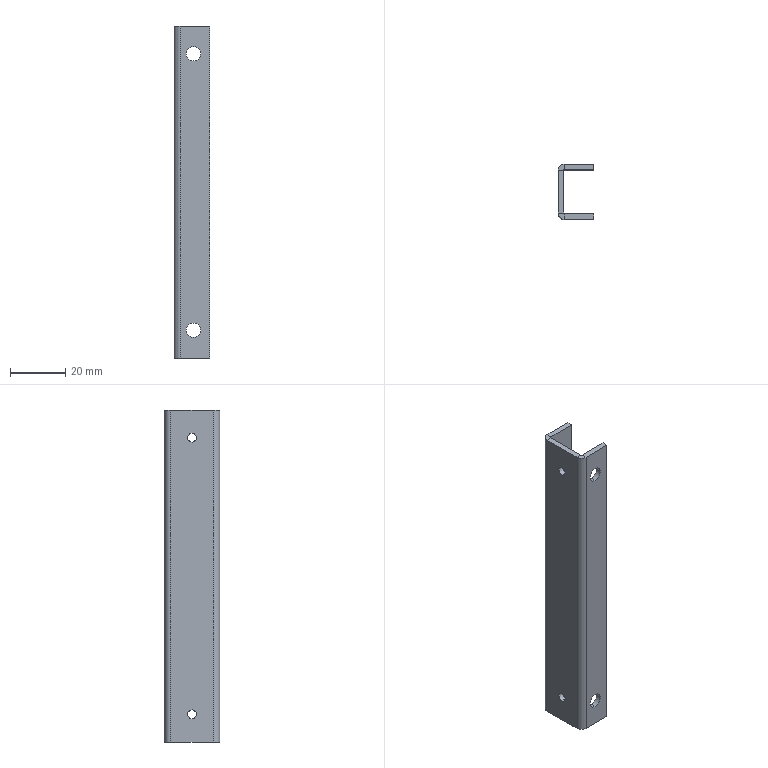Part | SolidWorks | features Cut 2, FlatPattern 1, SMBaseFlange 1, SheetMetal 1 | 1 solid | 34 faces | box 13 x 20 x 120 mm | volume 9610 mm3 | plane 18 | cylinder 16 | commonest cylinder face diameters 5.2 x8 3.2 x4 0.6 x2 4.6 x2
STEP:
#1=CARTESIAN_POINT('',(7.,18.,7.4));
#2=VERTEX_POINT('',#1);
#3=CARTESIAN_POINT('',(7.,18.,12.6));
#4=VERTEX_POINT('',#3);
#5=CARTESIAN_POINT('',(7.,18.,10.));
#6=DIRECTION('',(0.,1.,0.));
#7=DIRECTION('',(0.,0.,1.));
#8=AXIS2_PLACEMENT_3D('',#5,#6,#7);
#9=CIRCLE('',#8,2.6);
#10=EDGE_CURVE('',#2,#4,#9,.T.);
#11=ORIENTED_EDGE('',*,*,#10,.F.);
#12=CARTESIAN_POINT('',(7.,20.,7.4));
#13=VERTEX_POINT('',#12);
#14=CARTESIAN_POINT('',(7.,0.,7.4));
#15=DIRECTION('',(0.,1.,0.));
#16=VECTOR('',#15,1000.);
#17=LINE('',#14,#16);
#18=EDGE_CURVE('',#2,#13,#17,.T.);
#19=ORIENTED_EDGE('',*,*,#18,.T.);
#20=CARTESIAN_POINT('',(7.,20.,12.6));
#21=VERTEX_POINT('',#20);
#22=CARTESIAN_POINT('',(7.,20.,10.));
#23=DIRECTION('',(0.,1.,0.));
#24=DIRECTION('',(0.,0.,1.));
#25=AXIS2_PLACEMENT_3D('',#22,#23,#24);
#26=CIRCLE('',#25,2.6);
#27=EDGE_CURVE('',#13,#21,#26,.T.);
#28=ORIENTED_EDGE('',*,*,#27,.T.);
#29=CARTESIAN_POINT('',(7.,0.,12.6));
#30=DIRECTION('',(0.,1.,0.));
#31=VECTOR('',#30,1000.);
#32=LINE('',#29,#31);
#33=EDGE_CURVE('',#4,#21,#32,.T.);
#34=ORIENTED_EDGE('',*,*,#33,.F.);
#35=EDGE_LOOP('',(#11,#19,#28,#34));
#36=FACE_OUTER_BOUND('',#35,.T.);
#37=CARTESIAN_POINT('',(7.,0.,10.));
#38=DIRECTION('',(0.,1.,0.));
#39=DIRECTION('',(0.,0.,1.));
#40=AXIS2_PLACEMENT_3D('',#37,#38,#39);
#41=CYLINDRICAL_SURFACE('',#40,2.6);
#42=ADVANCED_FACE('',(#36),#41,.F.);
#43=CARTESIAN_POINT('',(7.,0.,7.4));
#44=VERTEX_POINT('',#43);
#45=CARTESIAN_POINT('',(7.,0.,12.6));
#46=VERTEX_POINT('',#45);
#47=CARTESIAN_POINT('',(7.,0.,10.));
#48=DIRECTION('',(0.,1.,0.));
#49=DIRECTION('',(0.,0.,1.));
#50=AXIS2_PLACEMENT_3D('',#47,#48,#49);
#51=CIRCLE('',#50,2.6);
#52=EDGE_CURVE('',#44,#46,#51,.T.);
#53=ORIENTED_EDGE('',*,*,#52,.F.);
#54=CARTESIAN_POINT('',(7.,2.,7.4));
#55=VERTEX_POINT('',#54);
#56=CARTESIAN_POINT('',(7.,0.,7.4));
#57=DIRECTION('',(0.,1.,0.));
#58=VECTOR('',#57,1000.);
#59=LINE('',#56,#58);
#60=EDGE_CURVE('',#44,#55,#59,.T.);
#61=ORIENTED_EDGE('',*,*,#60,.T.);
#62=CARTESIAN_POINT('',(7.,2.,12.6));
#63=VERTEX_POINT('',#62);
#64=CARTESIAN_POINT('',(7.,2.,10.));
#65=DIRECTION('',(0.,-1.,0.));
#66=DIRECTION('',(1.,0.,0.));
#67=AXIS2_PLACEMENT_3D('',#64,#65,#66);
#68=CIRCLE('',#67,2.6);
#69=EDGE_CURVE('',#63,#55,#68,.T.);
#70=ORIENTED_EDGE('',*,*,#69,.F.);
#71=CARTESIAN_POINT('',(7.,0.,12.6));
#72=DIRECTION('',(0.,1.,0.));
#73=VECTOR('',#72,1000.);
#74=LINE('',#71,#73);
#75=EDGE_CURVE('',#46,#63,#74,.T.);
#76=ORIENTED_EDGE('',*,*,#75,.F.);
#77=EDGE_LOOP('',(#53,#61,#70,#76));
#78=FACE_OUTER_BOUND('',#77,.T.);
#79=CARTESIAN_POINT('',(7.,0.,10.));
#80=DIRECTION('',(0.,1.,0.));
#81=DIRECTION('',(0.,0.,1.));
#82=AXIS2_PLACEMENT_3D('',#79,#80,#81);
#83=CYLINDRICAL_SURFACE('',#82,2.6);
#84=ADVANCED_FACE('',(#78),#83,.F.);
#85=CARTESIAN_POINT('',(7.,18.,107.4));
#86=VERTEX_POINT('',#85);
#87=CARTESIAN_POINT('',(7.,18.,112.6));
#88=VERTEX_POINT('',#87);
#89=CARTESIAN_POINT('',(7.,18.,110.));
#90=DIRECTION('',(0.,1.,0.));
#91=DIRECTION('',(0.,0.,1.));
#92=AXIS2_PLACEMENT_3D('',#89,#90,#91);
#93=CIRCLE('',#92,2.6);
#94=EDGE_CURVE('',#86,#88,#93,.T.);
#95=ORIENTED_EDGE('',*,*,#94,.F.);
#96=CARTESIAN_POINT('',(7.,20.,107.4));
#97=VERTEX_POINT('',#96);
#98=CARTESIAN_POINT('',(7.,0.,107.4));
#99=DIRECTION('',(0.,1.,0.));
#100=VECTOR('',#99,1000.);
#101=LINE('',#98,#100);
#102=EDGE_CURVE('',#86,#97,#101,.T.);
#103=ORIENTED_EDGE('',*,*,#102,.T.);
#104=CARTESIAN_POINT('',(7.,20.,112.6));
#105=VERTEX_POINT('',#104);
#106=CARTESIAN_POINT('',(7.,20.,110.));
#107=DIRECTION('',(0.,1.,0.));
#108=DIRECTION('',(0.,0.,1.));
#109=AXIS2_PLACEMENT_3D('',#106,#107,#108);
#110=CIRCLE('',#109,2.6);
#111=EDGE_CURVE('',#97,#105,#110,.T.);
#112=ORIENTED_EDGE('',*,*,#111,.T.);
#113=CARTESIAN_POINT('',(7.,0.,112.6));
#114=DIRECTION('',(0.,1.,0.));
#115=VECTOR('',#114,1000.);
#116=LINE('',#113,#115);
#117=EDGE_CURVE('',#88,#105,#116,.T.);
#118=ORIENTED_EDGE('',*,*,#117,.F.);
#119=EDGE_LOOP('',(#95,#103,#112,#118));
#120=FACE_OUTER_BOUND('',#119,.T.);
#121=CARTESIAN_POINT('',(7.,0.,110.));
#122=DIRECTION('',(0.,1.,0.));
#123=DIRECTION('',(0.,0.,1.));
#124=AXIS2_PLACEMENT_3D('',#121,#122,#123);
#125=CYLINDRICAL_SURFACE('',#124,2.6);
#126=ADVANCED_FACE('',(#120),#125,.F.);
#127=CARTESIAN_POINT('',(7.,0.,107.4));
#128=VERTEX_POINT('',#127);
#129=CARTESIAN_POINT('',(7.,0.,112.6));
#130=VERTEX_POINT('',#129);
#131=CARTESIAN_POINT('',(7.,0.,110.));
#132=DIRECTION('',(0.,1.,0.));
#133=DIRECTION('',(0.,0.,1.));
#134=AXIS2_PLACEMENT_3D('',#131,#132,#133);
#135=CIRCLE('',#134,2.6);
#136=EDGE_CURVE('',#128,#130,#135,.T.);
#137=ORIENTED_EDGE('',*,*,#136,.F.);
#138=CARTESIAN_POINT('',(7.,2.,107.4));
#139=VERTEX_POINT('',#138);
#140=CARTESIAN_POINT('',(7.,0.,107.4));
#141=DIRECTION('',(0.,1.,0.));
#142=VECTOR('',#141,1000.);
#143=LINE('',#140,#142);
#144=EDGE_CURVE('',#128,#139,#143,.T.);
#145=ORIENTED_EDGE('',*,*,#144,.T.);
#146=CARTESIAN_POINT('',(7.,2.,112.6));
#147=VERTEX_POINT('',#146);
#148=CARTESIAN_POINT('',(7.,2.,110.));
#149=DIRECTION('',(0.,-1.,0.));
#150=DIRECTION('',(1.,0.,0.));
#151=AXIS2_PLACEMENT_3D('',#148,#149,#150);
#152=CIRCLE('',#151,2.6);
#153=EDGE_CURVE('',#147,#139,#152,.T.);
#154=ORIENTED_EDGE('',*,*,#153,.F.);
#155=CARTESIAN_POINT('',(7.,0.,112.6));
#156=DIRECTION('',(0.,1.,0.));
#157=VECTOR('',#156,1000.);
#158=LINE('',#155,#157);
#159=EDGE_CURVE('',#130,#147,#158,.T.);
#160=ORIENTED_EDGE('',*,*,#159,.F.);
#161=EDGE_LOOP('',(#137,#145,#154,#160));
#162=FACE_OUTER_BOUND('',#161,.T.);
#163=CARTESIAN_POINT('',(7.,0.,110.));
#164=DIRECTION('',(0.,1.,0.));
#165=DIRECTION('',(0.,0.,1.));
#166=AXIS2_PLACEMENT_3D('',#163,#164,#165);
#167=CYLINDRICAL_SURFACE('',#166,2.6);
#168=ADVANCED_FACE('',(#162),#167,.F.);
#169=CARTESIAN_POINT('',(2.,10.,108.4));
#170=VERTEX_POINT('',#169);
#171=CARTESIAN_POINT('',(2.,10.,111.6));
#172=VERTEX_POINT('',#171);
#173=CARTESIAN_POINT('',(2.,10.,110.));
#174=DIRECTION('',(-1.,0.,0.));
#175=DIRECTION('',(0.,0.,1.));
#176=AXIS2_PLACEMENT_3D('',#173,#174,#175);
#177=CIRCLE('',#176,1.6);
#178=EDGE_CURVE('',#170,#172,#177,.T.);
#179=ORIENTED_EDGE('',*,*,#178,.F.);
#180=CARTESIAN_POINT('',(0.,10.,108.4));
#181=VERTEX_POINT('',#180);
#182=CARTESIAN_POINT('',(2.,10.,108.4));
#183=DIRECTION('',(-1.,0.,0.));
#184=VECTOR('',#183,1000.);
#185=LINE('',#182,#184);
#186=EDGE_CURVE('',#170,#181,#185,.T.);
#187=ORIENTED_EDGE('',*,*,#186,.T.);
#188=CARTESIAN_POINT('',(0.,10.,111.6));
#189=VERTEX_POINT('',#188);
#190=CARTESIAN_POINT('',(0.,10.,110.));
#191=DIRECTION('',(-1.,0.,0.));
#192=DIRECTION('',(0.,0.,1.));
#193=AXIS2_PLACEMENT_3D('',#190,#191,#192);
#194=CIRCLE('',#193,1.6);
#195=EDGE_CURVE('',#181,#189,#194,.T.);
#196=ORIENTED_EDGE('',*,*,#195,.T.);
#197=CARTESIAN_POINT('',(2.,10.,111.6));
#198=DIRECTION('',(-1.,0.,0.));
#199=VECTOR('',#198,1000.);
#200=LINE('',#197,#199);
#201=EDGE_CURVE('',#172,#189,#200,.T.);
#202=ORIENTED_EDGE('',*,*,#201,.F.);
#203=EDGE_LOOP('',(#179,#187,#196,#202));
#204=FACE_OUTER_BOUND('',#203,.T.);
#205=CARTESIAN_POINT('',(2.,10.,110.));
#206=DIRECTION('',(-1.,0.,0.));
#207=DIRECTION('',(0.,0.,1.));
#208=AXIS2_PLACEMENT_3D('',#205,#206,#207);
#209=CYLINDRICAL_SURFACE('',#208,1.6);
#210=ADVANCED_FACE('',(#204),#209,.F.);
#211=CARTESIAN_POINT('',(2.,10.,8.4));
#212=VERTEX_POINT('',#211);
#213=CARTESIAN_POINT('',(2.,10.,11.6));
#214=VERTEX_POINT('',#213);
#215=CARTESIAN_POINT('',(2.,10.,10.));
#216=DIRECTION('',(-1.,0.,0.));
#217=DIRECTION('',(0.,0.,1.));
#218=AXIS2_PLACEMENT_3D('',#215,#216,#217);
#219=CIRCLE('',#218,1.6);
#220=EDGE_CURVE('',#212,#214,#219,.T.);
#221=ORIENTED_EDGE('',*,*,#220,.F.);
#222=CARTESIAN_POINT('',(0.,10.,8.4));
#223=VERTEX_POINT('',#222);
#224=CARTESIAN_POINT('',(2.,10.,8.4));
#225=DIRECTION('',(-1.,0.,0.));
#226=VECTOR('',#225,1000.);
#227=LINE('',#224,#226);
#228=EDGE_CURVE('',#212,#223,#227,.T.);
#229=ORIENTED_EDGE('',*,*,#228,.T.);
#230=CARTESIAN_POINT('',(0.,10.,11.6));
#231=VERTEX_POINT('',#230);
#232=CARTESIAN_POINT('',(0.,10.,10.));
#233=DIRECTION('',(-1.,0.,0.));
#234=DIRECTION('',(0.,0.,1.));
#235=AXIS2_PLACEMENT_3D('',#232,#233,#234);
#236=CIRCLE('',#235,1.6);
#237=EDGE_CURVE('',#223,#231,#236,.T.);
#238=ORIENTED_EDGE('',*,*,#237,.T.);
#239=CARTESIAN_POINT('',(2.,10.,11.6));
#240=DIRECTION('',(-1.,0.,0.));
#241=VECTOR('',#240,1000.);
#242=LINE('',#239,#241);
#243=EDGE_CURVE('',#214,#231,#242,.T.);
#244=ORIENTED_EDGE('',*,*,#243,.F.);
#245=EDGE_LOOP('',(#221,#229,#238,#244));
#246=FACE_OUTER_BOUND('',#245,.T.);
#247=CARTESIAN_POINT('',(2.,10.,10.));
#248=DIRECTION('',(-1.,0.,0.));
#249=DIRECTION('',(0.,0.,1.));
#250=AXIS2_PLACEMENT_3D('',#247,#248,#249);
#251=CYLINDRICAL_SURFACE('',#250,1.6);
#252=ADVANCED_FACE('',(#246),#251,.F.);
#253=CARTESIAN_POINT('',(0.,2.3,120.));
#254=VERTEX_POINT('',#253);
#255=CARTESIAN_POINT('',(2.,2.3,120.));
#256=VERTEX_POINT('',#255);
#257=CARTESIAN_POINT('',(0.,2.3,120.));
#258=DIRECTION('',(1.,0.,0.));
#259=VECTOR('',#258,1000.);
#260=LINE('',#257,#259);
#261=EDGE_CURVE('',#254,#256,#260,.T.);
#262=ORIENTED_EDGE('',*,*,#261,.F.);
#263=CARTESIAN_POINT('',(2.3,0.,120.));
#264=VERTEX_POINT('',#263);
#265=CARTESIAN_POINT('',(2.3,2.3,120.));
#266=DIRECTION('',(0.,0.,-1.));
#267=DIRECTION('',(1.,0.,0.));
#268=AXIS2_PLACEMENT_3D('',#265,#266,#267);
#269=CIRCLE('',#268,2.3);
#270=EDGE_CURVE('',#264,#254,#269,.T.);
#271=ORIENTED_EDGE('',*,*,#270,.F.);
#272=CARTESIAN_POINT('',(2.3,2.,120.));
#273=VERTEX_POINT('',#272);
#274=CARTESIAN_POINT('',(2.3,2.,120.));
#275=DIRECTION('',(0.,-1.,0.));
#276=VECTOR('',#275,1000.);
#277=LINE('',#274,#276);
#278=EDGE_CURVE('',#273,#264,#277,.T.);
#279=ORIENTED_EDGE('',*,*,#278,.F.);
#280=CARTESIAN_POINT('',(2.3,2.3,120.));
#281=DIRECTION('',(0.,0.,-1.));
#282=DIRECTION('',(1.,0.,0.));
#283=AXIS2_PLACEMENT_3D('',#280,#281,#282);
#284=CIRCLE('',#283,0.3);
#285=EDGE_CURVE('',#273,#256,#284,.T.);
#286=ORIENTED_EDGE('',*,*,#285,.T.);
#287=EDGE_LOOP('',(#262,#271,#279,#286));
#288=FACE_OUTER_BOUND('',#287,.T.);
#289=CARTESIAN_POINT('',(0.,2.3,120.));
#290=DIRECTION('',(0.,0.,1.));
#291=DIRECTION('',(1.,0.,0.));
#292=AXIS2_PLACEMENT_3D('',#289,#290,#291);
#293=PLANE('',#292);
#294=ADVANCED_FACE('',(#288),#293,.T.);
#295=CARTESIAN_POINT('',(0.,17.7,120.));
#296=VERTEX_POINT('',#295);
#297=CARTESIAN_POINT('',(0.,0.,120.));
#298=DIRECTION('',(0.,1.,0.));
#299=VECTOR('',#298,1000.);
#300=LINE('',#297,#299);
#301=EDGE_CURVE('',#254,#296,#300,.T.);
#302=ORIENTED_EDGE('',*,*,#301,.F.);
#303=ORIENTED_EDGE('',*,*,#261,.T.);
#304=CARTESIAN_POINT('',(2.,17.7,120.));
#305=VERTEX_POINT('',#304);
#306=CARTESIAN_POINT('',(2.,0.,120.));
#307=DIRECTION('',(0.,1.,0.));
#308=VECTOR('',#307,1000.);
#309=LINE('',#306,#308);
#310=EDGE_CURVE('',#256,#305,#309,.T.);
#311=ORIENTED_EDGE('',*,*,#310,.T.);
#312=CARTESIAN_POINT('',(2.,17.7,120.));
#313=DIRECTION('',(-1.,0.,0.));
#314=VECTOR('',#313,1000.);
#315=LINE('',#312,#314);
#316=EDGE_CURVE('',#305,#296,#315,.T.);
#317=ORIENTED_EDGE('',*,*,#316,.T.);
#318=EDGE_LOOP('',(#302,#303,#311,#317));
#319=FACE_OUTER_BOUND('',#318,.T.);
#320=CARTESIAN_POINT('',(2.3,2.,120.));
#321=DIRECTION('',(0.,0.,1.));
#322=DIRECTION('',(1.,0.,0.));
#323=AXIS2_PLACEMENT_3D('',#320,#321,#322);
#324=PLANE('',#323);
#325=ADVANCED_FACE('',(#319),#324,.T.);
#326=CARTESIAN_POINT('',(2.3,0.,0.));
#327=VERTEX_POINT('',#326);
#328=CARTESIAN_POINT('',(2.3,2.,0.));
#329=VERTEX_POINT('',#328);
#330=CARTESIAN_POINT('',(2.3,0.,0.));
#331=DIRECTION('',(0.,1.,0.));
#332=VECTOR('',#331,1000.);
#333=LINE('',#330,#332);
#334=EDGE_CURVE('',#327,#329,#333,.T.);
#335=ORIENTED_EDGE('',*,*,#334,.F.);
#336=CARTESIAN_POINT('',(0.,2.3,0.));
#337=VERTEX_POINT('',#336);
#338=CARTESIAN_POINT('',(2.3,2.3,0.));
#339=DIRECTION('',(0.,0.,-1.));
#340=DIRECTION('',(1.,0.,0.));
#341=AXIS2_PLACEMENT_3D('',#338,#339,#340);
#342=CIRCLE('',#341,2.3);
#343=EDGE_CURVE('',#327,#337,#342,.T.);
#344=ORIENTED_EDGE('',*,*,#343,.T.);
#345=CARTESIAN_POINT('',(2.,2.3,0.));
#346=VERTEX_POINT('',#345);
#347=CARTESIAN_POINT('',(2.,2.3,0.));
#348=DIRECTION('',(-1.,0.,0.));
#349=VECTOR('',#348,1000.);
#350=LINE('',#347,#349);
#351=EDGE_CURVE('',#346,#337,#350,.T.);
#352=ORIENTED_EDGE('',*,*,#351,.F.);
#353=CARTESIAN_POINT('',(2.3,2.3,0.));
#354=DIRECTION('',(0.,0.,-1.));
#355=DIRECTION('',(1.,0.,0.));
#356=AXIS2_PLACEMENT_3D('',#353,#354,#355);
#357=CIRCLE('',#356,0.3);
#358=EDGE_CURVE('',#329,#346,#357,.T.);
#359=ORIENTED_EDGE('',*,*,#358,.F.);
#360=EDGE_LOOP('',(#335,#344,#352,#359));
#361=FACE_OUTER_BOUND('',#360,.T.);
#362=CARTESIAN_POINT('',(2.3,0.,0.));
#363=DIRECTION('',(0.,0.,-1.));
#364=DIRECTION('',(-1.,0.,0.));
#365=AXIS2_PLACEMENT_3D('',#362,#363,#364);
#366=PLANE('',#365);
#367=ADVANCED_FACE('',(#361),#366,.T.);
#368=CARTESIAN_POINT('',(13.,0.,0.));
#369=VERTEX_POINT('',#368);
#370=CARTESIAN_POINT('',(13.,0.,0.));
#371=DIRECTION('',(-1.,0.,0.));
#372=VECTOR('',#371,1000.);
#373=LINE('',#370,#372);
#374=EDGE_CURVE('',#369,#327,#373,.T.);
#375=ORIENTED_EDGE('',*,*,#374,.T.);
#376=ORIENTED_EDGE('',*,*,#334,.T.);
#377=CARTESIAN_POINT('',(13.,2.,0.));
#378=VERTEX_POINT('',#377);
#379=CARTESIAN_POINT('',(13.,2.,0.));
#380=DIRECTION('',(-1.,0.,0.));
#381=VECTOR('',#380,1000.);
#382=LINE('',#379,#381);
#383=EDGE_CURVE('',#378,#329,#382,.T.);
#384=ORIENTED_EDGE('',*,*,#383,.F.);
#385=CARTESIAN_POINT('',(13.,2.,0.));
#386=DIRECTION('',(0.,-1.,0.));
#387=VECTOR('',#386,1000.);
#388=LINE('',#385,#387);
#389=EDGE_CURVE('',#378,#369,#388,.T.);
#390=ORIENTED_EDGE('',*,*,#389,.T.);
#391=EDGE_LOOP('',(#375,#376,#384,#390));
#392=FACE_OUTER_BOUND('',#391,.T.);
#393=CARTESIAN_POINT('',(2.,2.3,0.));
#394=DIRECTION('',(0.,0.,-1.));
#395=DIRECTION('',(-1.,0.,0.));
#396=AXIS2_PLACEMENT_3D('',#393,#394,#395);
#397=PLANE('',#396);
#398=ADVANCED_FACE('',(#392),#397,.T.);
#399=CARTESIAN_POINT('',(2.3,20.,120.));
#400=VERTEX_POINT('',#399);
#401=CARTESIAN_POINT('',(2.3,18.,120.));
#402=VERTEX_POINT('',#401);
#403=CARTESIAN_POINT('',(2.3,20.,120.));
#404=DIRECTION('',(0.,-1.,0.));
#405=VECTOR('',#404,1000.);
#406=LINE('',#403,#405);
#407=EDGE_CURVE('',#400,#402,#406,.T.);
#408=ORIENTED_EDGE('',*,*,#407,.F.);
#409=CARTESIAN_POINT('',(2.3,17.7,120.));
#410=DIRECTION('',(0.,0.,-1.));
#411=DIRECTION('',(1.,0.,0.));
#412=AXIS2_PLACEMENT_3D('',#409,#410,#411);
#413=CIRCLE('',#412,2.3);
#414=EDGE_CURVE('',#296,#400,#413,.T.);
#415=ORIENTED_EDGE('',*,*,#414,.F.);
#416=ORIENTED_EDGE('',*,*,#316,.F.);
#417=CARTESIAN_POINT('',(2.3,17.7,120.));
#418=DIRECTION('',(0.,0.,-1.));
#419=DIRECTION('',(1.,0.,0.));
#420=AXIS2_PLACEMENT_3D('',#417,#418,#419);
#421=CIRCLE('',#420,0.3);
#422=EDGE_CURVE('',#305,#402,#421,.T.);
#423=ORIENTED_EDGE('',*,*,#422,.T.);
#424=EDGE_LOOP('',(#408,#415,#416,#423));
#425=FACE_OUTER_BOUND('',#424,.T.);
#426=CARTESIAN_POINT('',(2.3,20.,120.));
#427=DIRECTION('',(0.,0.,1.));
#428=DIRECTION('',(1.,0.,0.));
#429=AXIS2_PLACEMENT_3D('',#426,#427,#428);
#430=PLANE('',#429);
#431=ADVANCED_FACE('',(#425),#430,.T.);
#432=CARTESIAN_POINT('',(13.,20.,120.));
#433=VERTEX_POINT('',#432);
#434=CARTESIAN_POINT('',(0.,20.,120.));
#435=DIRECTION('',(1.,0.,0.));
#436=VECTOR('',#435,1000.);
#437=LINE('',#434,#436);
#438=EDGE_CURVE('',#400,#433,#437,.T.);
#439=ORIENTED_EDGE('',*,*,#438,.F.);
#440=ORIENTED_EDGE('',*,*,#407,.T.);
#441=CARTESIAN_POINT('',(13.,18.,120.));
#442=VERTEX_POINT('',#441);
#443=CARTESIAN_POINT('',(0.,18.,120.));
#444=DIRECTION('',(1.,0.,0.));
#445=VECTOR('',#444,1000.);
#446=LINE('',#443,#445);
#447=EDGE_CURVE('',#402,#442,#446,.T.);
#448=ORIENTED_EDGE('',*,*,#447,.T.);
#449=CARTESIAN_POINT('',(13.,20.,120.));
#450=DIRECTION('',(0.,-1.,0.));
#451=VECTOR('',#450,1000.);
#452=LINE('',#449,#451);
#453=EDGE_CURVE('',#433,#442,#452,.T.);
#454=ORIENTED_EDGE('',*,*,#453,.F.);
#455=EDGE_LOOP('',(#439,#440,#448,#454));
#456=FACE_OUTER_BOUND('',#455,.T.);
#457=CARTESIAN_POINT('',(2.,17.7,120.));
#458=DIRECTION('',(0.,0.,1.));
#459=DIRECTION('',(1.,0.,0.));
#460=AXIS2_PLACEMENT_3D('',#457,#458,#459);
#461=PLANE('',#460);
#462=ADVANCED_FACE('',(#456),#461,.T.);
#463=CARTESIAN_POINT('',(0.,17.7,0.));
#464=VERTEX_POINT('',#463);
#465=CARTESIAN_POINT('',(2.,17.7,0.));
#466=VERTEX_POINT('',#465);
#467=CARTESIAN_POINT('',(0.,17.7,0.));
#468=DIRECTION('',(1.,0.,0.));
#469=VECTOR('',#468,1000.);
#470=LINE('',#467,#469);
#471=EDGE_CURVE('',#464,#466,#470,.T.);
#472=ORIENTED_EDGE('',*,*,#471,.F.);
#473=CARTESIAN_POINT('',(2.3,20.,0.));
#474=VERTEX_POINT('',#473);
#475=CARTESIAN_POINT('',(2.3,17.7,0.));
#476=DIRECTION('',(0.,0.,-1.));
#477=DIRECTION('',(1.,0.,0.));
#478=AXIS2_PLACEMENT_3D('',#475,#476,#477);
#479=CIRCLE('',#478,2.3);
#480=EDGE_CURVE('',#464,#474,#479,.T.);
#481=ORIENTED_EDGE('',*,*,#480,.T.);
#482=CARTESIAN_POINT('',(2.3,18.,0.));
#483=VERTEX_POINT('',#482);
#484=CARTESIAN_POINT('',(2.3,18.,0.));
#485=DIRECTION('',(0.,1.,0.));
#486=VECTOR('',#485,1000.);
#487=LINE('',#484,#486);
#488=EDGE_CURVE('',#483,#474,#487,.T.);
#489=ORIENTED_EDGE('',*,*,#488,.F.);
#490=CARTESIAN_POINT('',(2.3,17.7,0.));
#491=DIRECTION('',(0.,0.,-1.));
#492=DIRECTION('',(1.,0.,0.));
#493=AXIS2_PLACEMENT_3D('',#490,#491,#492);
#494=CIRCLE('',#493,0.3);
#495=EDGE_CURVE('',#466,#483,#494,.T.);
#496=ORIENTED_EDGE('',*,*,#495,.F.);
#497=EDGE_LOOP('',(#472,#481,#489,#496));
#498=FACE_OUTER_BOUND('',#497,.T.);
#499=CARTESIAN_POINT('',(0.,17.7,0.));
#500=DIRECTION('',(0.,0.,-1.));
#501=DIRECTION('',(-1.,0.,0.));
#502=AXIS2_PLACEMENT_3D('',#499,#500,#501);
#503=PLANE('',#502);
#504=ADVANCED_FACE('',(#498),#503,.T.);
#505=CARTESIAN_POINT('',(0.,0.,0.));
#506=DIRECTION('',(0.,1.,0.));
#507=VECTOR('',#506,1000.);
#508=LINE('',#505,#507);
#509=EDGE_CURVE('',#337,#464,#508,.T.);
#510=ORIENTED_EDGE('',*,*,#509,.T.);
#511=ORIENTED_EDGE('',*,*,#471,.T.);
#512=CARTESIAN_POINT('',(2.,0.,0.));
#513=DIRECTION('',(0.,1.,0.));
#514=VECTOR('',#513,1000.);
#515=LINE('',#512,#514);
#516=EDGE_CURVE('',#346,#466,#515,.T.);
#517=ORIENTED_EDGE('',*,*,#516,.F.);
#518=ORIENTED_EDGE('',*,*,#351,.T.);
#519=EDGE_LOOP('',(#510,#511,#517,#518));
#520=FACE_OUTER_BOUND('',#519,.T.);
#521=CARTESIAN_POINT('',(2.3,18.,0.));
#522=DIRECTION('',(0.,0.,-1.));
#523=DIRECTION('',(-1.,0.,0.));
#524=AXIS2_PLACEMENT_3D('',#521,#522,#523);
#525=PLANE('',#524);
#526=ADVANCED_FACE('',(#520),#525,.T.);
#527=CARTESIAN_POINT('',(7.,18.,10.));
#528=DIRECTION('',(0.,1.,0.));
#529=DIRECTION('',(0.,0.,1.));
#530=AXIS2_PLACEMENT_3D('',#527,#528,#529);
#531=CIRCLE('',#530,2.6);
#532=EDGE_CURVE('',#4,#2,#531,.T.);
#533=ORIENTED_EDGE('',*,*,#532,.T.);
#534=ORIENTED_EDGE('',*,*,#10,.T.);
#535=EDGE_LOOP('',(#533,#534));
#536=FACE_BOUND('',#535,.T.);
#537=CARTESIAN_POINT('',(7.,18.,110.));
#538=DIRECTION('',(0.,1.,0.));
#539=DIRECTION('',(0.,0.,1.));
#540=AXIS2_PLACEMENT_3D('',#537,#538,#539);
#541=CIRCLE('',#540,2.6);
#542=EDGE_CURVE('',#88,#86,#541,.T.);
#543=ORIENTED_EDGE('',*,*,#542,.T.);
#544=ORIENTED_EDGE('',*,*,#94,.T.);
#545=EDGE_LOOP('',(#543,#544));
#546=FACE_BOUND('',#545,.T.);
#547=CARTESIAN_POINT('',(13.,18.,0.));
#548=VERTEX_POINT('',#547);
#549=CARTESIAN_POINT('',(0.,18.,0.));
#550=DIRECTION('',(1.,0.,0.));
#551=VECTOR('',#550,1000.);
#552=LINE('',#549,#551);
#553=EDGE_CURVE('',#483,#548,#552,.T.);
#554=ORIENTED_EDGE('',*,*,#553,.T.);
#555=CARTESIAN_POINT('',(13.,18.,120.));
#556=DIRECTION('',(0.,0.,-1.));
#557=VECTOR('',#556,1000.);
#558=LINE('',#555,#557);
#559=EDGE_CURVE('',#442,#548,#558,.T.);
#560=ORIENTED_EDGE('',*,*,#559,.F.);
#561=ORIENTED_EDGE('',*,*,#447,.F.);
#562=CARTESIAN_POINT('',(2.3,18.,120.));
#563=DIRECTION('',(0.,0.,-1.));
#564=VECTOR('',#563,1000.);
#565=LINE('',#562,#564);
#566=EDGE_CURVE('',#402,#483,#565,.T.);
#567=ORIENTED_EDGE('',*,*,#566,.T.);
#568=EDGE_LOOP('',(#554,#560,#561,#567));
#569=FACE_OUTER_BOUND('',#568,.T.);
#570=CARTESIAN_POINT('',(0.,18.,120.));
#571=DIRECTION('',(0.,1.,0.));
#572=DIRECTION('',(0.,0.,1.));
#573=AXIS2_PLACEMENT_3D('',#570,#571,#572);
#574=PLANE('',#573);
#575=ADVANCED_FACE('',(#536,#546,#569),#574,.F.);
#576=CARTESIAN_POINT('',(13.,20.,0.));
#577=VERTEX_POINT('',#576);
#578=CARTESIAN_POINT('',(13.,20.,0.));
#579=DIRECTION('',(0.,-1.,0.));
#580=VECTOR('',#579,1000.);
#581=LINE('',#578,#580);
#582=EDGE_CURVE('',#577,#548,#581,.T.);
#583=ORIENTED_EDGE('',*,*,#582,.F.);
#584=CARTESIAN_POINT('',(13.,20.,120.));
#585=DIRECTION('',(0.,0.,-1.));
#586=VECTOR('',#585,1000.);
#587=LINE('',#584,#586);
#588=EDGE_CURVE('',#433,#577,#587,.T.);
#589=ORIENTED_EDGE('',*,*,#588,.F.);
#590=ORIENTED_EDGE('',*,*,#453,.T.);
#591=ORIENTED_EDGE('',*,*,#559,.T.);
#592=EDGE_LOOP('',(#583,#589,#590,#591));
#593=FACE_OUTER_BOUND('',#592,.T.);
#594=CARTESIAN_POINT('',(13.,20.,120.));
#595=DIRECTION('',(1.,0.,0.));
#596=DIRECTION('',(0.,0.,-1.));
#597=AXIS2_PLACEMENT_3D('',#594,#595,#596);
#598=PLANE('',#597);
#599=ADVANCED_FACE('',(#593),#598,.T.);
#600=CARTESIAN_POINT('',(7.,20.,10.));
#601=DIRECTION('',(0.,1.,0.));
#602=DIRECTION('',(0.,0.,1.));
#603=AXIS2_PLACEMENT_3D('',#600,#601,#602);
#604=CIRCLE('',#603,2.6);
#605=EDGE_CURVE('',#21,#13,#604,.T.);
#606=ORIENTED_EDGE('',*,*,#605,.F.);
#607=ORIENTED_EDGE('',*,*,#27,.F.);
#608=EDGE_LOOP('',(#606,#607));
#609=FACE_BOUND('',#608,.T.);
#610=CARTESIAN_POINT('',(7.,20.,110.));
#611=DIRECTION('',(0.,1.,0.));
#612=DIRECTION('',(0.,0.,1.));
#613=AXIS2_PLACEMENT_3D('',#610,#611,#612);
#614=CIRCLE('',#613,2.6);
#615=EDGE_CURVE('',#105,#97,#614,.T.);
#616=ORIENTED_EDGE('',*,*,#615,.F.);
#617=ORIENTED_EDGE('',*,*,#111,.F.);
#618=EDGE_LOOP('',(#616,#617));
#619=FACE_BOUND('',#618,.T.);
#620=CARTESIAN_POINT('',(0.,20.,0.));
#621=DIRECTION('',(1.,0.,0.));
#622=VECTOR('',#621,1000.);
#623=LINE('',#620,#622);
#624=EDGE_CURVE('',#474,#577,#623,.T.);
#625=ORIENTED_EDGE('',*,*,#624,.F.);
#626=CARTESIAN_POINT('',(2.3,20.,120.));
#627=DIRECTION('',(0.,0.,-1.));
#628=VECTOR('',#627,1000.);
#629=LINE('',#626,#628);
#630=EDGE_CURVE('',#400,#474,#629,.T.);
#631=ORIENTED_EDGE('',*,*,#630,.F.);
#632=ORIENTED_EDGE('',*,*,#438,.T.);
#633=ORIENTED_EDGE('',*,*,#588,.T.);
#634=EDGE_LOOP('',(#625,#631,#632,#633));
#635=FACE_OUTER_BOUND('',#634,.T.);
#636=CARTESIAN_POINT('',(0.,20.,120.));
#637=DIRECTION('',(0.,1.,0.));
#638=DIRECTION('',(0.,0.,1.));
#639=AXIS2_PLACEMENT_3D('',#636,#637,#638);
#640=PLANE('',#639);
#641=ADVANCED_FACE('',(#609,#619,#635),#640,.T.);
#642=ORIENTED_EDGE('',*,*,#480,.F.);
#643=CARTESIAN_POINT('',(0.,17.7,120.));
#644=DIRECTION('',(0.,0.,-1.));
#645=VECTOR('',#644,1000.);
#646=LINE('',#643,#645);
#647=EDGE_CURVE('',#296,#464,#646,.T.);
#648=ORIENTED_EDGE('',*,*,#647,.F.);
#649=ORIENTED_EDGE('',*,*,#414,.T.);
#650=ORIENTED_EDGE('',*,*,#630,.T.);
#651=EDGE_LOOP('',(#642,#648,#649,#650));
#652=FACE_OUTER_BOUND('',#651,.T.);
#653=CARTESIAN_POINT('',(2.3,17.7,120.));
#654=DIRECTION('',(0.,0.,-1.));
#655=DIRECTION('',(-1.,0.,0.));
#656=AXIS2_PLACEMENT_3D('',#653,#654,#655);
#657=CYLINDRICAL_SURFACE('',#656,2.3);
#658=ADVANCED_FACE('',(#652),#657,.T.);
#659=CARTESIAN_POINT('',(0.,10.,110.));
#660=DIRECTION('',(-1.,0.,0.));
#661=DIRECTION('',(0.,0.,1.));
#662=AXIS2_PLACEMENT_3D('',#659,#660,#661);
#663=CIRCLE('',#662,1.6);
#664=EDGE_CURVE('',#189,#181,#663,.T.);
#665=ORIENTED_EDGE('',*,*,#664,.F.);
#666=ORIENTED_EDGE('',*,*,#195,.F.);
#667=EDGE_LOOP('',(#665,#666));
#668=FACE_BOUND('',#667,.T.);
#669=CARTESIAN_POINT('',(0.,10.,10.));
#670=DIRECTION('',(-1.,0.,0.));
#671=DIRECTION('',(0.,0.,1.));
#672=AXIS2_PLACEMENT_3D('',#669,#670,#671);
#673=CIRCLE('',#672,1.6);
#674=EDGE_CURVE('',#231,#223,#673,.T.);
#675=ORIENTED_EDGE('',*,*,#674,.F.);
#676=ORIENTED_EDGE('',*,*,#237,.F.);
#677=EDGE_LOOP('',(#675,#676));
#678=FACE_BOUND('',#677,.T.);
#679=ORIENTED_EDGE('',*,*,#509,.F.);
#680=CARTESIAN_POINT('',(0.,2.3,120.));
#681=DIRECTION('',(0.,0.,-1.));
#682=VECTOR('',#681,1000.);
#683=LINE('',#680,#682);
#684=EDGE_CURVE('',#254,#337,#683,.T.);
#685=ORIENTED_EDGE('',*,*,#684,.F.);
#686=ORIENTED_EDGE('',*,*,#301,.T.);
#687=ORIENTED_EDGE('',*,*,#647,.T.);
#688=EDGE_LOOP('',(#679,#685,#686,#687));
#689=FACE_OUTER_BOUND('',#688,.T.);
#690=CARTESIAN_POINT('',(0.,0.,120.));
#691=DIRECTION('',(-1.,0.,0.));
#692=DIRECTION('',(0.,0.,1.));
#693=AXIS2_PLACEMENT_3D('',#690,#691,#692);
#694=PLANE('',#693);
#695=ADVANCED_FACE('',(#668,#678,#689),#694,.T.);
#696=ORIENTED_EDGE('',*,*,#343,.F.);
#697=CARTESIAN_POINT('',(2.3,0.,120.));
#698=DIRECTION('',(0.,0.,-1.));
#699=VECTOR('',#698,1000.);
#700=LINE('',#697,#699);
#701=EDGE_CURVE('',#264,#327,#700,.T.);
#702=ORIENTED_EDGE('',*,*,#701,.F.);
#703=ORIENTED_EDGE('',*,*,#270,.T.);
#704=ORIENTED_EDGE('',*,*,#684,.T.);
#705=EDGE_LOOP('',(#696,#702,#703,#704));
#706=FACE_OUTER_BOUND('',#705,.T.);
#707=CARTESIAN_POINT('',(2.3,2.3,120.));
#708=DIRECTION('',(0.,0.,-1.));
#709=DIRECTION('',(-1.,0.,0.));
#710=AXIS2_PLACEMENT_3D('',#707,#708,#709);
#711=CYLINDRICAL_SURFACE('',#710,2.3);
#712=ADVANCED_FACE('',(#706),#711,.T.);
#713=CARTESIAN_POINT('',(7.,0.,10.));
#714=DIRECTION('',(0.,1.,0.));
#715=DIRECTION('',(0.,0.,1.));
#716=AXIS2_PLACEMENT_3D('',#713,#714,#715);
#717=CIRCLE('',#716,2.6);
#718=EDGE_CURVE('',#46,#44,#717,.T.);
#719=ORIENTED_EDGE('',*,*,#718,.T.);
#720=ORIENTED_EDGE('',*,*,#52,.T.);
#721=EDGE_LOOP('',(#719,#720));
#722=FACE_BOUND('',#721,.T.);
#723=CARTESIAN_POINT('',(7.,0.,110.));
#724=DIRECTION('',(0.,1.,0.));
#725=DIRECTION('',(0.,0.,1.));
#726=AXIS2_PLACEMENT_3D('',#723,#724,#725);
#727=CIRCLE('',#726,2.6);
#728=EDGE_CURVE('',#130,#128,#727,.T.);
#729=ORIENTED_EDGE('',*,*,#728,.T.);
#730=ORIENTED_EDGE('',*,*,#136,.T.);
#731=EDGE_LOOP('',(#729,#730));
#732=FACE_BOUND('',#731,.T.);
#733=ORIENTED_EDGE('',*,*,#374,.F.);
#734=CARTESIAN_POINT('',(13.,0.,120.));
#735=VERTEX_POINT('',#734);
#736=CARTESIAN_POINT('',(13.,0.,120.));
#737=DIRECTION('',(0.,0.,-1.));
#738=VECTOR('',#737,1000.);
#739=LINE('',#736,#738);
#740=EDGE_CURVE('',#735,#369,#739,.T.);
#741=ORIENTED_EDGE('',*,*,#740,.F.);
#742=CARTESIAN_POINT('',(13.,0.,120.));
#743=DIRECTION('',(-1.,0.,0.));
#744=VECTOR('',#743,1000.);
#745=LINE('',#742,#744);
#746=EDGE_CURVE('',#735,#264,#745,.T.);
#747=ORIENTED_EDGE('',*,*,#746,.T.);
#748=ORIENTED_EDGE('',*,*,#701,.T.);
#749=EDGE_LOOP('',(#733,#741,#747,#748));
#750=FACE_OUTER_BOUND('',#749,.T.);
#751=CARTESIAN_POINT('',(13.,0.,120.));
#752=DIRECTION('',(0.,-1.,0.));
#753=DIRECTION('',(1.,0.,0.));
#754=AXIS2_PLACEMENT_3D('',#751,#752,#753);
#755=PLANE('',#754);
#756=ADVANCED_FACE('',(#722,#732,#750),#755,.T.);
#757=ORIENTED_EDGE('',*,*,#389,.F.);
#758=CARTESIAN_POINT('',(13.,2.,120.));
#759=VERTEX_POINT('',#758);
#760=CARTESIAN_POINT('',(13.,2.,120.));
#761=DIRECTION('',(0.,0.,-1.));
#762=VECTOR('',#761,1000.);
#763=LINE('',#760,#762);
#764=EDGE_CURVE('',#759,#378,#763,.T.);
#765=ORIENTED_EDGE('',*,*,#764,.F.);
#766=CARTESIAN_POINT('',(13.,2.,120.));
#767=DIRECTION('',(0.,-1.,0.));
#768=VECTOR('',#767,1000.);
#769=LINE('',#766,#768);
#770=EDGE_CURVE('',#759,#735,#769,.T.);
#771=ORIENTED_EDGE('',*,*,#770,.T.);
#772=ORIENTED_EDGE('',*,*,#740,.T.);
#773=EDGE_LOOP('',(#757,#765,#771,#772));
#774=FACE_OUTER_BOUND('',#773,.T.);
#775=CARTESIAN_POINT('',(13.,2.,120.));
#776=DIRECTION('',(1.,0.,0.));
#777=DIRECTION('',(0.,0.,-1.));
#778=AXIS2_PLACEMENT_3D('',#775,#776,#777);
#779=PLANE('',#778);
#780=ADVANCED_FACE('',(#774),#779,.T.);
#781=ORIENTED_EDGE('',*,*,#69,.T.);
#782=CARTESIAN_POINT('',(7.,2.,10.));
#783=DIRECTION('',(0.,-1.,0.));
#784=DIRECTION('',(1.,0.,0.));
#785=AXIS2_PLACEMENT_3D('',#782,#783,#784);
#786=CIRCLE('',#785,2.6);
#787=EDGE_CURVE('',#55,#63,#786,.T.);
#788=ORIENTED_EDGE('',*,*,#787,.T.);
#789=EDGE_LOOP('',(#781,#788));
#790=FACE_BOUND('',#789,.T.);
#791=ORIENTED_EDGE('',*,*,#153,.T.);
#792=CARTESIAN_POINT('',(7.,2.,110.));
#793=DIRECTION('',(0.,-1.,0.));
#794=DIRECTION('',(1.,0.,0.));
#795=AXIS2_PLACEMENT_3D('',#792,#793,#794);
#796=CIRCLE('',#795,2.6);
#797=EDGE_CURVE('',#139,#147,#796,.T.);
#798=ORIENTED_EDGE('',*,*,#797,.T.);
#799=EDGE_LOOP('',(#791,#798));
#800=FACE_BOUND('',#799,.T.);
#801=ORIENTED_EDGE('',*,*,#383,.T.);
#802=CARTESIAN_POINT('',(2.3,2.,120.));
#803=DIRECTION('',(0.,0.,-1.));
#804=VECTOR('',#803,1000.);
#805=LINE('',#802,#804);
#806=EDGE_CURVE('',#273,#329,#805,.T.);
#807=ORIENTED_EDGE('',*,*,#806,.F.);
#808=CARTESIAN_POINT('',(13.,2.,120.));
#809=DIRECTION('',(-1.,0.,0.));
#810=VECTOR('',#809,1000.);
#811=LINE('',#808,#810);
#812=EDGE_CURVE('',#759,#273,#811,.T.);
#813=ORIENTED_EDGE('',*,*,#812,.F.);
#814=ORIENTED_EDGE('',*,*,#764,.T.);
#815=EDGE_LOOP('',(#801,#807,#813,#814));
#816=FACE_OUTER_BOUND('',#815,.T.);
#817=CARTESIAN_POINT('',(13.,2.,120.));
#818=DIRECTION('',(0.,-1.,0.));
#819=DIRECTION('',(1.,0.,0.));
#820=AXIS2_PLACEMENT_3D('',#817,#818,#819);
#821=PLANE('',#820);
#822=ADVANCED_FACE('',(#790,#800,#816),#821,.F.);
#823=ORIENTED_EDGE('',*,*,#358,.T.);
#824=CARTESIAN_POINT('',(2.,2.3,120.));
#825=DIRECTION('',(0.,0.,-1.));
#826=VECTOR('',#825,1000.);
#827=LINE('',#824,#826);
#828=EDGE_CURVE('',#256,#346,#827,.T.);
#829=ORIENTED_EDGE('',*,*,#828,.F.);
#830=ORIENTED_EDGE('',*,*,#285,.F.);
#831=ORIENTED_EDGE('',*,*,#806,.T.);
#832=EDGE_LOOP('',(#823,#829,#830,#831));
#833=FACE_OUTER_BOUND('',#832,.T.);
#834=CARTESIAN_POINT('',(2.3,2.3,120.));
#835=DIRECTION('',(0.,0.,-1.));
#836=DIRECTION('',(-1.,0.,0.));
#837=AXIS2_PLACEMENT_3D('',#834,#835,#836);
#838=CYLINDRICAL_SURFACE('',#837,0.3);
#839=ADVANCED_FACE('',(#833),#838,.F.);
#840=CARTESIAN_POINT('',(2.,10.,110.));
#841=DIRECTION('',(-1.,0.,0.));
#842=DIRECTION('',(0.,0.,1.));
#843=AXIS2_PLACEMENT_3D('',#840,#841,#842);
#844=CIRCLE('',#843,1.6);
#845=EDGE_CURVE('',#172,#170,#844,.T.);
#846=ORIENTED_EDGE('',*,*,#845,.T.);
#847=ORIENTED_EDGE('',*,*,#178,.T.);
#848=EDGE_LOOP('',(#846,#847));
#849=FACE_BOUND('',#848,.T.);
#850=CARTESIAN_POINT('',(2.,10.,10.));
#851=DIRECTION('',(-1.,0.,0.));
#852=DIRECTION('',(0.,0.,1.));
#853=AXIS2_PLACEMENT_3D('',#850,#851,#852);
#854=CIRCLE('',#853,1.6);
#855=EDGE_CURVE('',#214,#212,#854,.T.);
#856=ORIENTED_EDGE('',*,*,#855,.T.);
#857=ORIENTED_EDGE('',*,*,#220,.T.);
#858=EDGE_LOOP('',(#856,#857));
#859=FACE_BOUND('',#858,.T.);
#860=ORIENTED_EDGE('',*,*,#516,.T.);
#861=CARTESIAN_POINT('',(2.,17.7,120.));
#862=DIRECTION('',(0.,0.,-1.));
#863=VECTOR('',#862,1000.);
#864=LINE('',#861,#863);
#865=EDGE_CURVE('',#305,#466,#864,.T.);
#866=ORIENTED_EDGE('',*,*,#865,.F.);
#867=ORIENTED_EDGE('',*,*,#310,.F.);
#868=ORIENTED_EDGE('',*,*,#828,.T.);
#869=EDGE_LOOP('',(#860,#866,#867,#868));
#870=FACE_OUTER_BOUND('',#869,.T.);
#871=CARTESIAN_POINT('',(2.,0.,120.));
#872=DIRECTION('',(-1.,0.,0.));
#873=DIRECTION('',(0.,0.,1.));
#874=AXIS2_PLACEMENT_3D('',#871,#872,#873);
#875=PLANE('',#874);
#876=ADVANCED_FACE('',(#849,#859,#870),#875,.F.);
#877=ORIENTED_EDGE('',*,*,#495,.T.);
#878=ORIENTED_EDGE('',*,*,#566,.F.);
#879=ORIENTED_EDGE('',*,*,#422,.F.);
#880=ORIENTED_EDGE('',*,*,#865,.T.);
#881=EDGE_LOOP('',(#877,#878,#879,#880));
#882=FACE_OUTER_BOUND('',#881,.T.);
#883=CARTESIAN_POINT('',(2.3,17.7,120.));
#884=DIRECTION('',(0.,0.,-1.));
#885=DIRECTION('',(-1.,0.,0.));
#886=AXIS2_PLACEMENT_3D('',#883,#884,#885);
#887=CYLINDRICAL_SURFACE('',#886,0.3);
#888=ADVANCED_FACE('',(#882),#887,.F.);
#889=ORIENTED_EDGE('',*,*,#812,.T.);
#890=ORIENTED_EDGE('',*,*,#278,.T.);
#891=ORIENTED_EDGE('',*,*,#746,.F.);
#892=ORIENTED_EDGE('',*,*,#770,.F.);
#893=EDGE_LOOP('',(#889,#890,#891,#892));
#894=FACE_OUTER_BOUND('',#893,.T.);
#895=CARTESIAN_POINT('',(2.3,17.7,120.));
#896=DIRECTION('',(0.,0.,1.));
#897=DIRECTION('',(1.,0.,0.));
#898=AXIS2_PLACEMENT_3D('',#895,#896,#897);
#899=PLANE('',#898);
#900=ADVANCED_FACE('',(#894),#899,.T.);
#901=ORIENTED_EDGE('',*,*,#553,.F.);
#902=ORIENTED_EDGE('',*,*,#488,.T.);
#903=ORIENTED_EDGE('',*,*,#624,.T.);
#904=ORIENTED_EDGE('',*,*,#582,.T.);
#905=EDGE_LOOP('',(#901,#902,#903,#904));
#906=FACE_OUTER_BOUND('',#905,.T.);
#907=CARTESIAN_POINT('',(2.3,17.7,0.));
#908=DIRECTION('',(0.,0.,1.));
#909=DIRECTION('',(1.,0.,0.));
#910=AXIS2_PLACEMENT_3D('',#907,#908,#909);
#911=PLANE('',#910);
#912=ADVANCED_FACE('',(#906),#911,.F.);
#913=ORIENTED_EDGE('',*,*,#228,.F.);
#914=ORIENTED_EDGE('',*,*,#855,.F.);
#915=ORIENTED_EDGE('',*,*,#243,.T.);
#916=ORIENTED_EDGE('',*,*,#674,.T.);
#917=EDGE_LOOP('',(#913,#914,#915,#916));
#918=FACE_OUTER_BOUND('',#917,.T.);
#919=CARTESIAN_POINT('',(2.,10.,10.));
#920=DIRECTION('',(-1.,0.,0.));
#921=DIRECTION('',(0.,0.,1.));
#922=AXIS2_PLACEMENT_3D('',#919,#920,#921);
#923=CYLINDRICAL_SURFACE('',#922,1.6);
#924=ADVANCED_FACE('',(#918),#923,.F.);
#925=ORIENTED_EDGE('',*,*,#186,.F.);
#926=ORIENTED_EDGE('',*,*,#845,.F.);
#927=ORIENTED_EDGE('',*,*,#201,.T.);
#928=ORIENTED_EDGE('',*,*,#664,.T.);
#929=EDGE_LOOP('',(#925,#926,#927,#928));
#930=FACE_OUTER_BOUND('',#929,.T.);
#931=CARTESIAN_POINT('',(2.,10.,110.));
#932=DIRECTION('',(-1.,0.,0.));
#933=DIRECTION('',(0.,0.,1.));
#934=AXIS2_PLACEMENT_3D('',#931,#932,#933);
#935=CYLINDRICAL_SURFACE('',#934,1.6);
#936=ADVANCED_FACE('',(#930),#935,.F.);
#937=ORIENTED_EDGE('',*,*,#144,.F.);
#938=ORIENTED_EDGE('',*,*,#728,.F.);
#939=ORIENTED_EDGE('',*,*,#159,.T.);
#940=ORIENTED_EDGE('',*,*,#797,.F.);
#941=EDGE_LOOP('',(#937,#938,#939,#940));
#942=FACE_OUTER_BOUND('',#941,.T.);
#943=CARTESIAN_POINT('',(7.,0.,110.));
#944=DIRECTION('',(0.,1.,0.));
#945=DIRECTION('',(0.,0.,1.));
#946=AXIS2_PLACEMENT_3D('',#943,#944,#945);
#947=CYLINDRICAL_SURFACE('',#946,2.6);
#948=ADVANCED_FACE('',(#942),#947,.F.);
#949=ORIENTED_EDGE('',*,*,#102,.F.);
#950=ORIENTED_EDGE('',*,*,#542,.F.);
#951=ORIENTED_EDGE('',*,*,#117,.T.);
#952=ORIENTED_EDGE('',*,*,#615,.T.);
#953=EDGE_LOOP('',(#949,#950,#951,#952));
#954=FACE_OUTER_BOUND('',#953,.T.);
#955=CARTESIAN_POINT('',(7.,0.,110.));
#956=DIRECTION('',(0.,1.,0.));
#957=DIRECTION('',(0.,0.,1.));
#958=AXIS2_PLACEMENT_3D('',#955,#956,#957);
#959=CYLINDRICAL_SURFACE('',#958,2.6);
#960=ADVANCED_FACE('',(#954),#959,.F.);
#961=ORIENTED_EDGE('',*,*,#60,.F.);
#962=ORIENTED_EDGE('',*,*,#718,.F.);
#963=ORIENTED_EDGE('',*,*,#75,.T.);
#964=ORIENTED_EDGE('',*,*,#787,.F.);
#965=EDGE_LOOP('',(#961,#962,#963,#964));
#966=FACE_OUTER_BOUND('',#965,.T.);
#967=CARTESIAN_POINT('',(7.,0.,10.));
#968=DIRECTION('',(0.,1.,0.));
#969=DIRECTION('',(0.,0.,1.));
#970=AXIS2_PLACEMENT_3D('',#967,#968,#969);
#971=CYLINDRICAL_SURFACE('',#970,2.6);
#972=ADVANCED_FACE('',(#966),#971,.F.);
#973=ORIENTED_EDGE('',*,*,#18,.F.);
#974=ORIENTED_EDGE('',*,*,#532,.F.);
#975=ORIENTED_EDGE('',*,*,#33,.T.);
#976=ORIENTED_EDGE('',*,*,#605,.T.);
#977=EDGE_LOOP('',(#973,#974,#975,#976));
#978=FACE_OUTER_BOUND('',#977,.T.);
#979=CARTESIAN_POINT('',(7.,0.,10.));
#980=DIRECTION('',(0.,1.,0.));
#981=DIRECTION('',(0.,0.,1.));
#982=AXIS2_PLACEMENT_3D('',#979,#980,#981);
#983=CYLINDRICAL_SURFACE('',#982,2.6);
#984=ADVANCED_FACE('',(#978),#983,.F.);
#985=CLOSED_SHELL('',(#42,#84,#126,#168,#210,#252,#294,#325,#367,#398,#431,#462,#504,#526,#575,#599,#641,#658,#695,#712,#756,#780,#822,#839,#876,#888,#900,#912,#924,#936,#948,#960,#972,#984));
#986=MANIFOLD_SOLID_BREP('',#985);
#987=CARTESIAN_POINT('',(0.,0.,0.));
#988=DIRECTION('',(0.,0.,1.));
#989=DIRECTION('',(1.,0.,0.));
#990=AXIS2_PLACEMENT_3D('',#987,#988,#989);
#991=(LENGTH_UNIT()NAMED_UNIT(*)SI_UNIT(.MILLI.,.METRE.));
#992=UNCERTAINTY_MEASURE_WITH_UNIT(LENGTH_MEASURE(0.00001),#991,'','');
#993=(NAMED_UNIT(*)PLANE_ANGLE_UNIT()SI_UNIT($,.RADIAN.));
#994=(NAMED_UNIT(*)SI_UNIT($,.STERADIAN.)SOLID_ANGLE_UNIT());
#995=(GEOMETRIC_REPRESENTATION_CONTEXT(3)GLOBAL_UNCERTAINTY_ASSIGNED_CONTEXT((#992))GLOBAL_UNIT_ASSIGNED_CONTEXT((#991,#993,#994))REPRESENTATION_CONTEXT('',''));
#996=ADVANCED_BREP_SHAPE_REPRESENTATION('',(#986,#990),#995);